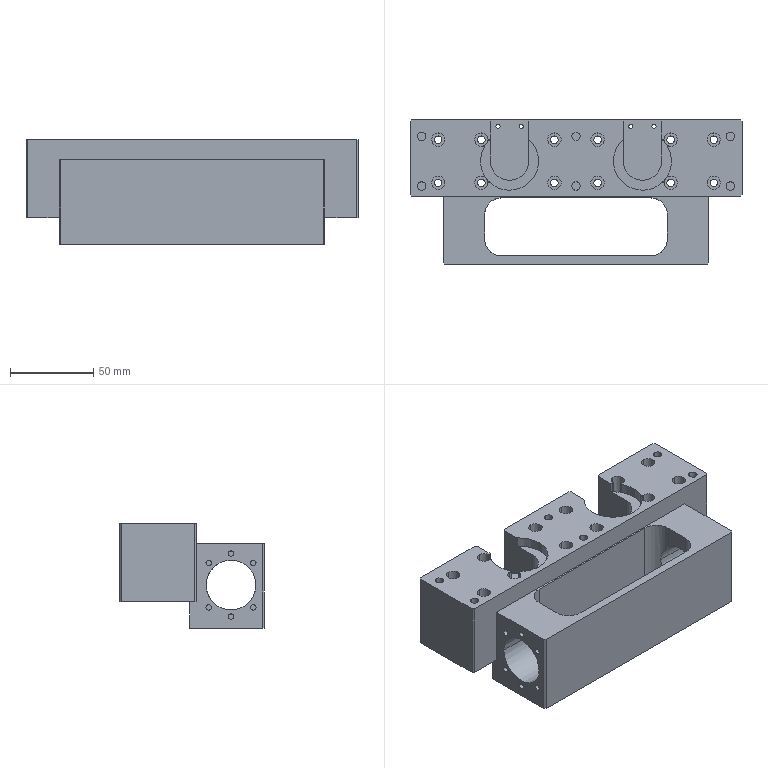CAM job | NX | 3-axis milling, drilling | part box 200 x 87 x 63 mm | stock box 206 x 93 x 64 mm
Tools:
number,name,description,diameter,corner_radius,flute_length,length,flutes
1,D63,Milling Tool-5 Parameters,63.0,0.0,50.0,75.0,2
20,D20,Milling Tool-5 Parameters,20.0,0.0,50.0,75.0,2
11,D10JING,Milling Tool-5 Parameters,10.0,0.0,50.0,75.0,2
7,D6A45,Milling Tool-5 Parameters,6.0,0.0,3.0,3.0,2
12,2.5ZT,Drilling Tool,2.5,0.0,35.0,50.0,2
13,M3,Milling Tool-5 Parameters,2.5,0.0,30.0,30.0,4
15,5.2ZT,Drilling Tool,5.1,0.0,35.0,50.0,2
16,M6,Milling Tool-5 Parameters,5.0,0.0,30.0,30.0,4
14,4.5ZT,Drilling Tool,4.5,0.0,35.0,50.0,2
6,D6,Milling Tool-5 Parameters,6.0,0.0,50.0,75.0,2
Operations:
program,operation,operation_type,tool,method,geometry_group,spindle_rpm,surface_speed,feed_per_tooth,feed_cut,feed_plunge,cut_length_mm,path_length_mm,cut_time_min,machine_time_min
1-65-90-205毛胚,FLOOR_WALL,VolumeBased25DMillingOperation,D63,METHOD,A,6500.0,1286.0,0.0962,1250.0,100.0,886.797,940.797,0.7094,0.7148
1-65-90-205毛胚,CAVITY_MILL,CavityMilling,D20,METHOD,A,7000.0,439.0,0.1571,2200.0,1000.0,149436.705,157041.503,70.598,71.738
1-65-90-205毛胚,DRILLING_COPY_1,Operation,D6A45,METHOD,A,3000.0,56.0,0.0333,200.0,0.0,101.2,891.978,0.506,0.5851
1-65-90-205毛胚,DRILLING_COPY_1_COPY,Operation,2.5ZT,METHOD,A,2000.0,15.0,0.0375,150.0,0.0,69.004,371.712,0.46,0.4903
1-65-90-205毛胚,DRILLING_COPY_1_COPY_COPY,Operation,M3,METHOD,A,200.0,1.0,0.125,100.0,0.0,62.0,357.704,0.62,0.6496
1-65-90-205毛胚,DRILLING_COPY_1_COPY_COPY_1,Operation,5.2ZT,METHOD,A,2000.0,15.0,0.0375,150.0,0.0,147.193,645.932,0.9813,1.031
1-65-90-205毛胚,DRILLING_COPY_1_COPY_COPY_1_COPY,Operation,M6,METHOD,A,200.0,3.0,0.125,100.0,0.0,108.0,567.546,1.08,1.126
1-65-90-205毛胚,DRILLING_COPY_1_COPY_COPY_1_COPY_1,Operation,4.5ZT,METHOD,A,2000.0,15.0,0.0375,150.0,0.0,634.223,1685.203,4.228,4.333
1-65-90-205毛胚,ZLEVEL_PROFILE_COPY_1,ZLevelMilling,D10JING,METHOD,A,7000.0,87.0,0.1071,1500.0,1000.0,8727.632,14533.221,6.46,7.041
1-65-90-205毛胚,ZLEVEL_PROFILE_COPY_COPY_1_COPY_COPY_COPY_1,ZLevelMilling,D10JING,METHOD,A,7000.0,219.0,0.0714,1000.0,100.0,3630.418,4128.55,3.63,3.68
1-65-90-205毛胚,FLOOR_WALL_1_COPY_1,VolumeBased25DMillingOperation,D10JING,METHOD,A,7000.0,87.0,0.0714,1000.0,100.0,2278.759,3276.695,2.279,2.391
1-65-90-205毛胚,HOLE_MILLING,CylinderMilling,D6,METHOD,A,7000.0,131.0,0.0714,1000.0,100.0,8038.93,9493.454,8.039,8.184
1-65-90-205毛胚,ZLEVEL_PROFILE_COPY_1_COPY_COPY_COPY_COPY_2_COPY,ZLevelMilling,D6A45,METHOD,A,7000.0,131.0,0.0714,1000.0,1000.0,1007.624,3359.768,1.008,1.243
1-65-90-205毛胚,ZLEVEL_PROFILE_COPY_1_COPY_COPY_COPY_COPY_2_COPY_COPY,ZLevelMilling,D6A45,METHOD,A,7000.0,131.0,0.0714,1000.0,1000.0,412.044,618.574,0.412,0.4327